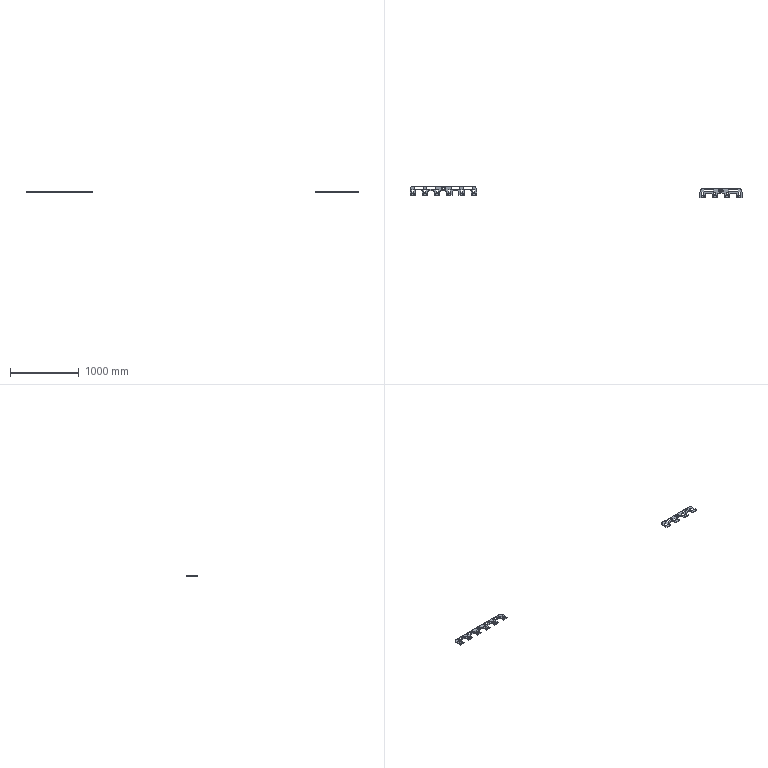NC program | NX | posted with a generic post | part box 4825 x 168.213 x 13 mm
Lines 4335 to 5402 of 9095:
(HOLE_MILLING , TOOL : D6)
N8620 T06 M6
N8622 G54
N8624 G17 G0 G90 X-10.715 Y58.869 S9500 M3
N8626 G43 Z30. H6
N8628 Z0.5
N8630 G94 G3 X-10.215 Y58.369 R0.5 F1400.
N8632 X-9.715 Y58.869 R0.5
N8634 X-9.715 Y58.869 Z0. I-1. J0.
N8636 X-9.715 Y58.869 Z-0.5 I-1. J0.
N8638 X-9.715 Y58.869 Z-1. I-1. J0.
N8640 X-9.715 Y58.869 Z-1.5 I-1. J0.
N8642 X-9.715 Y58.869 Z-2. I-1. J0.
N8644 X-9.715 Y58.869 Z-2.5 I-1. J0.
N8646 X-9.715 Y58.869 Z-3. I-1. J0.
N8648 X-9.715 Y58.869 Z-3.5 I-1. J0.
N8650 X-9.715 Y58.869 Z-4. I-1. J0.
N8652 X-9.715 Y58.869 Z-4.5 I-1. J0.
N8654 X-10.406 Y59.82 Z-4.6 R1.
N8656 X-11.666 Y59.178 R1.
N8658 X-10.406 Y59.82 R-1.
N8660 X-11.036 Y59.499 R0.5
N8662 X-10.715 Y58.869 R0.5
N8664 G0 Z30.
N8666 X-25.869 Y43.715
N8668 Z0.5
N8670 G3 X-25.369 Y43.215 R0.5
N8672 X-24.869 Y43.715 R0.5
N8674 X-24.869 Y43.715 Z0. I-1. J0.
N8676 X-24.869 Y43.715 Z-0.5 I-1. J0.
N8678 X-24.869 Y43.715 Z-1. I-1. J0.
N8680 X-24.869 Y43.715 Z-1.5 I-1. J0.
N8682 X-24.869 Y43.715 Z-2. I-1. J0.
N8684 X-24.869 Y43.715 Z-2.5 I-1. J0.
N8686 X-24.869 Y43.715 Z-3. I-1. J0.
N8688 X-24.869 Y43.715 Z-3.5 I-1. J0.
N8690 X-24.869 Y43.715 Z-4. I-1. J0.
N8692 X-24.869 Y43.715 Z-4.5 I-1. J0.
N8694 X-25.56 Y44.666 Z-4.6 R1.
N8696 X-26.82 Y44.024 R1.
N8698 X-25.56 Y44.666 R-1.
N8700 X-26.19 Y44.345 R0.5
N8702 X-25.869 Y43.715 R0.5
N8704 G0 Z30.
N8706 Y22.285
N8708 Z0.5
N8710 G3 X-25.369 Y21.785 R0.5
N8712 X-24.869 Y22.285 R0.5
N8714 X-24.869 Y22.285 Z0. I-1. J0.
N8716 X-24.869 Y22.285 Z-0.5 I-1. J0.
N8718 X-24.869 Y22.285 Z-1. I-1. J0.
N8720 X-24.869 Y22.285 Z-1.5 I-1. J0.
N8722 X-24.869 Y22.285 Z-2. I-1. J0.
N8724 X-24.869 Y22.285 Z-2.5 I-1. J0.
N8726 X-24.869 Y22.285 Z-3. I-1. J0.
N8728 X-24.869 Y22.285 Z-3.5 I-1. J0.
N8730 X-24.869 Y22.285 Z-4. I-1. J0.
N8732 X-24.869 Y22.285 Z-4.5 I-1. J0.
N8734 X-25.56 Y23.236 Z-4.6 R1.
N8736 X-26.82 Y22.594 R1.
N8738 X-25.56 Y23.236 R-1.
N8740 X-26.19 Y22.915 R0.5
N8742 X-25.869 Y22.285 R0.5
N8744 G0 Z30.
N8746 X-10.715 Y7.131
N8748 Z0.5
N8750 G3 X-10.215 Y6.631 R0.5
N8752 X-9.715 Y7.131 R0.5
N8754 X-9.715 Y7.131 Z0. I-1. J0.
N8756 X-9.715 Y7.131 Z-0.5 I-1. J0.
N8758 X-9.715 Y7.131 Z-1. I-1. J0.
N8760 X-9.715 Y7.131 Z-1.5 I-1. J0.
N8762 X-9.715 Y7.131 Z-2. I-1. J0.
N8764 X-9.715 Y7.131 Z-2.5 I-1. J0.
N8766 X-9.715 Y7.131 Z-3. I-1. J0.
N8768 X-9.715 Y7.131 Z-3.5 I-1. J0.
N8770 X-9.715 Y7.131 Z-4. I-1. J0.
N8772 X-9.715 Y7.131 Z-4.5 I-1. J0.
N8774 X-10.406 Y8.082 Z-4.6 R1.
N8776 X-11.666 Y7.44 R1.
N8778 X-10.406 Y8.082 R-1.
N8780 X-11.036 Y7.761 R0.5
N8782 X-10.715 Y7.131 R0.5
N8784 G0 Z30.
N8786 X10.715
N8788 Z0.5
N8790 G3 X11.215 Y6.631 R0.5
N8792 X11.715 Y7.131 R0.5
N8794 X11.715 Y7.131 Z0. I-1. J0.
N8796 X11.715 Y7.131 Z-0.5 I-1. J0.
N8798 X11.715 Y7.131 Z-1. I-1. J0.
N8800 X11.715 Y7.131 Z-1.5 I-1. J0.
N8802 X11.715 Y7.131 Z-2. I-1. J0.
N8804 X11.715 Y7.131 Z-2.5 I-1. J0.
N8806 X11.715 Y7.131 Z-3. I-1. J0.
N8808 X11.715 Y7.131 Z-3.5 I-1. J0.
N8810 X11.715 Y7.131 Z-4. I-1. J0.
N8812 X11.715 Y7.131 Z-4.5 I-1. J0.
N8814 X11.024 Y8.082 Z-4.6 R1.
N8816 X9.764 Y7.44 R1.
N8818 X11.024 Y8.082 R-1.
N8820 X10.394 Y7.761 R0.5
N8822 X10.715 Y7.131 R0.5
N8824 G0 Z30.
N8826 X25.869 Y22.285
N8828 Z0.5
N8830 G3 X26.369 Y21.785 R0.5
N8832 X26.869 Y22.285 R0.5
N8834 X26.869 Y22.285 Z0. I-1. J0.
N8836 X26.869 Y22.285 Z-0.5 I-1. J0.
N8838 X26.869 Y22.285 Z-1. I-1. J0.
N8840 X26.869 Y22.285 Z-1.5 I-1. J0.
N8842 X26.869 Y22.285 Z-2. I-1. J0.
N8844 X26.869 Y22.285 Z-2.5 I-1. J0.
N8846 X26.869 Y22.285 Z-3. I-1. J0.
N8848 X26.869 Y22.285 Z-3.5 I-1. J0.
N8850 X26.869 Y22.285 Z-4. I-1. J0.
N8852 X26.869 Y22.285 Z-4.5 I-1. J0.
N8854 X26.178 Y23.236 Z-4.6 R1.
N8856 X24.918 Y22.594 R1.
N8858 X26.178 Y23.236 R-1.
N8860 X25.548 Y22.915 R0.5
N8862 X25.869 Y22.285 R0.5
N8864 G0 Z30.
N8866 Y43.715
N8868 Z0.5
N8870 G3 X26.369 Y43.215 R0.5
N8872 X26.869 Y43.715 R0.5
N8874 X26.869 Y43.715 Z0. I-1. J0.
N8876 X26.869 Y43.715 Z-0.5 I-1. J0.
N8878 X26.869 Y43.715 Z-1. I-1. J0.
N8880 X26.869 Y43.715 Z-1.5 I-1. J0.
N8882 X26.869 Y43.715 Z-2. I-1. J0.
N8884 X26.869 Y43.715 Z-2.5 I-1. J0.
N8886 X26.869 Y43.715 Z-3. I-1. J0.
N8888 X26.869 Y43.715 Z-3.5 I-1. J0.
N8890 X26.869 Y43.715 Z-4. I-1. J0.
N8892 X26.869 Y43.715 Z-4.5 I-1. J0.
N8894 X26.178 Y44.666 Z-4.6 R1.
N8896 X24.918 Y44.024 R1.
N8898 X26.178 Y44.666 R-1.
N8900 X25.548 Y44.345 R0.5
N8902 X25.869 Y43.715 R0.5
N8904 G0 Z30.
N8906 X10.715 Y58.869
N8908 Z0.5
N8910 G3 X11.215 Y58.369 R0.5
N8912 X11.715 Y58.869 R0.5
N8914 X11.715 Y58.869 Z0. I-1. J0.
N8916 X11.715 Y58.869 Z-0.5 I-1. J0.
N8918 X11.715 Y58.869 Z-1. I-1. J0.
N8920 X11.715 Y58.869 Z-1.5 I-1. J0.
N8922 X11.715 Y58.869 Z-2. I-1. J0.
N8924 X11.715 Y58.869 Z-2.5 I-1. J0.
N8926 X11.715 Y58.869 Z-3. I-1. J0.
N8928 X11.715 Y58.869 Z-3.5 I-1. J0.
N8930 X11.715 Y58.869 Z-4. I-1. J0.
N8932 X11.715 Y58.869 Z-4.5 I-1. J0.
N8934 X11.024 Y59.82 Z-4.6 R1.
N8936 X9.764 Y59.178 R1.
N8938 X11.024 Y59.82 R-1.
N8940 X10.394 Y59.499 R0.5
N8942 X10.715 Y58.869 R0.5
N8944 G0 Z30.
(ZLEVEL_PROFILE_COPY_1 , TOOL : D6)
N8946 X276.421 Y-19.8
N8948 Z-0.591
N8950 G1 Y-20.997 F1000.
N8952 X276.484 Y-21.
N8954 X278.7 F1650.
N8956 Y-18.784
N8958 X278.697 Y-18.721
N8960 X277.5
N8962 G0 X276.421 Y-19.8 Z-1.182
N8964 G1 Y-20.997 F1000.
N8966 X276.484 Y-21.
N8968 X278.7 F1650.
N8970 Y-18.784
N8972 X278.697 Y-18.721
N8974 X277.5
N8976 G0 X276.421 Y-19.8 Z-1.773
N8978 G1 Y-20.997 F1000.
N8980 X276.484 Y-21.
N8982 X278.7 F1650.
N8984 Y-18.784
N8986 X278.697 Y-18.721
N8988 X277.5
N8990 G0 X276.421 Y-19.8 Z-2.364
N8992 G1 Y-20.997 F1000.
N8994 X276.484 Y-21.
N8996 X278.7 F1650.
N8998 Y-18.784
N9000 X278.697 Y-18.721
N9002 X277.5
N9004 G0 X276.421 Y-19.8 Z-2.955
N9006 G1 Y-20.997 F1000.
N9008 X276.484 Y-21.
N9010 X278.7 F1650.
N9012 Y-18.784
N9014 X278.697 Y-18.721
N9016 X277.5
N9018 G0 X276.421 Y-19.8 Z-3.545
N9020 G1 Y-20.997 F1000.
N9022 X276.484 Y-21.
N9024 X278.7 F1650.
N9026 Y-18.784
N9028 X278.697 Y-18.721
N9030 X277.5
N9032 G0 X276.421 Y-19.8 Z-4.136
N9034 G1 Y-20.997 F1000.
N9036 X276.484 Y-21.
N9038 X278.7 F1650.
N9040 Y-18.784
N9042 X278.697 Y-18.721
N9044 X277.5
N9046 G0 X276.421 Y-19.8 Z-4.727
N9048 G1 Y-20.997 F1000.
N9050 X276.484 Y-21.
N9052 X278.7 F1650.
N9054 Y-18.784
N9056 X278.697 Y-18.721
N9058 X277.5
N9060 G0 X276.421 Y-19.8 Z-5.318
N9062 G1 Y-20.997 F1000.
N9064 X276.484 Y-21.
N9066 X278.7 F1650.
N9068 Y-18.784
N9070 X278.697 Y-18.721
N9072 X277.5
N9074 G0 X276.421 Y-19.8 Z-5.909
N9076 G1 Y-20.997 F1000.
N9078 X276.484 Y-21.
N9080 X278.7 F1650.
N9082 Y-18.784
N9084 X278.697 Y-18.721
N9086 X277.5
N9088 G0 X276.421 Y-19.8 Z-6.5
N9090 G1 Y-20.997 F1000.
N9092 X276.484 Y-21.
N9094 X278.7 F1650.
N9096 Y-18.784
N9098 X278.697 Y-18.721
N9100 X277.5
N9102 G0 X276.421 Y-19.8 Z-7.091
N9104 G1 Y-20.997 F1000.
N9106 X276.484 Y-21.
N9108 X278.7 F1650.
N9110 Y-18.784
N9112 X278.697 Y-18.721
N9114 X277.5
N9116 G0 X276.421 Y-19.8 Z-7.682
N9118 G1 Y-20.997 F1000.
N9120 X276.484 Y-21.
N9122 X278.7 F1650.
N9124 Y-18.784
N9126 X278.697 Y-18.721
N9128 X277.5
N9130 G0 X276.416 Y-19.8 Z-8.273
N9132 G1 Y-20.997 F1000.
N9134 X276.479 Y-21.
N9136 X278.7 F1650.
N9138 Y-18.783
N9140 X278.697 Y-18.72
N9142 X277.5
N9144 G0 X276.416 Y-19.8 Z-8.864
N9146 G1 Y-20.997 F1000.
N9148 X276.479 Y-21.
N9150 X278.7 F1650.
N9152 Y-18.783
N9154 X278.697 Y-18.72
N9156 X277.5
N9158 G0 X276.416 Y-19.8 Z-9.455
N9160 G1 Y-20.997 F1000.
N9162 X276.479 Y-21.
N9164 X278.7 F1650.
N9166 Y-18.783
N9168 X278.697 Y-18.72
N9170 X277.5
N9172 G0 X276.416 Y-19.8 Z-10.045
N9174 G1 Y-20.997 F1000.
N9176 X276.479 Y-21.
N9178 X278.7 F1650.
N9180 Y-18.783
N9182 X278.697 Y-18.72
N9184 X277.5
N9186 G0 X276.416 Y-19.8 Z-10.636
N9188 G1 Y-20.997 F1000.
N9190 X276.479 Y-21.
N9192 X278.7 F1650.
N9194 Y-18.783
N9196 X278.697 Y-18.72
N9198 X277.5
N9200 G0 X276.416 Y-19.8 Z-11.227
N9202 G1 Y-20.997 F1000.
N9204 X276.479 Y-21.
N9206 X278.7 F1650.
N9208 Y-18.783
N9210 X278.697 Y-18.72
N9212 X277.5
N9214 G0 X276.416 Y-19.8 Z-11.818
N9216 G1 Y-20.997 F1000.
N9218 X276.479 Y-21.
N9220 X278.7 F1650.
N9222 Y-18.783
N9224 X278.697 Y-18.72
N9226 X277.5
N9228 G0 X276.416 Y-19.8 Z-12.409
N9230 G1 Y-20.997 F1000.
N9232 X276.479 Y-21.
N9234 X278.7 F1650.
N9236 Y-18.783
N9238 X278.697 Y-18.72
N9240 X277.5
N9242 G0 X276.416 Y-19.8 Z-13.
N9244 G1 Y-20.997 F1000.
N9246 X276.479 Y-21.
N9248 X278.7 F1650.
N9250 Y-18.783
N9252 X278.697 Y-18.72
N9254 X277.5
N9256 G0 Z30.
N9258 Y10.721
N9260 Z-0.591
N9262 G1 X278.697 F1000.
N9264 X278.7 Y10.784
N9266 Y13. F1650.
N9268 X276.484
N9270 X276.421 Y12.997
N9272 Y11.8
N9274 G0 X277.5 Y10.721 Z-1.182
N9276 G1 X278.697 F1000.
N9278 X278.7 Y10.784
N9280 Y13. F1650.
N9282 X276.484
N9284 X276.421 Y12.997
N9286 Y11.8
N9288 G0 X277.5 Y10.721 Z-1.773
N9290 G1 X278.697 F1000.
N9292 X278.7 Y10.784
N9294 Y13. F1650.
N9296 X276.484
N9298 X276.421 Y12.997
N9300 Y11.8
N9302 G0 X277.5 Y10.721 Z-2.364
N9304 G1 X278.697 F1000.
N9306 X278.7 Y10.784
N9308 Y13. F1650.
N9310 X276.484
N9312 X276.421 Y12.997
N9314 Y11.8
N9316 G0 X277.5 Y10.721 Z-2.955
N9318 G1 X278.697 F1000.
N9320 X278.7 Y10.784
N9322 Y13. F1650.
N9324 X276.484
N9326 X276.421 Y12.997
N9328 Y11.8
N9330 G0 X277.5 Y10.721 Z-3.545
N9332 G1 X278.697 F1000.
N9334 X278.7 Y10.784
N9336 Y13. F1650.
N9338 X276.484
N9340 X276.421 Y12.997
N9342 Y11.8
N9344 G0 X277.5 Y10.721 Z-4.136
N9346 G1 X278.697 F1000.
N9348 X278.7 Y10.784
N9350 Y13. F1650.
N9352 X276.484
N9354 X276.421 Y12.997
N9356 Y11.8
N9358 G0 X277.5 Y10.721 Z-4.727
N9360 G1 X278.697 F1000.
N9362 X278.7 Y10.784
N9364 Y13. F1650.
N9366 X276.484
N9368 X276.421 Y12.997
N9370 Y11.8
N9372 G0 X277.5 Y10.721 Z-5.318
N9374 G1 X278.697 F1000.
N9376 X278.7 Y10.784
N9378 Y13. F1650.
N9380 X276.484
N9382 X276.421 Y12.997
N9384 Y11.8
N9386 G0 X277.5 Y10.721 Z-5.909
N9388 G1 X278.697 F1000.
N9390 X278.7 Y10.784
N9392 Y13. F1650.
N9394 X276.484
N9396 X276.421 Y12.997
N9398 Y11.8
N9400 G0 X277.5 Y10.721 Z-6.5
N9402 G1 X278.697 F1000.
N9404 X278.7 Y10.784
N9406 Y13. F1650.
N9408 X276.484
N9410 X276.421 Y12.997
N9412 Y11.8
N9414 G0 X277.5 Y10.721 Z-7.091
N9416 G1 X278.697 F1000.
N9418 X278.7 Y10.784
N9420 Y13. F1650.
N9422 X276.484
N9424 X276.421 Y12.997
N9426 Y11.8
N9428 G0 X277.5 Y10.721 Z-7.682
N9430 G1 X278.697 F1000.
N9432 X278.7 Y10.784
N9434 Y13. F1650.
N9436 X276.484
N9438 X276.421 Y12.997
N9440 Y11.8
N9442 G0 X277.5 Y10.722 Z-8.273
N9444 G1 X278.697 F1000.
N9446 X278.7 Y10.785
N9448 Y12.991 F1650.
N9450 Y13.
N9452 X276.492
N9454 X276.429 Y12.997
N9456 Y11.8
N9458 G0 X277.5 Y10.722 Z-8.864
N9460 G1 X278.697 F1000.
N9462 X278.7 Y10.785
N9464 Y12.991 F1650.
N9466 Y13.
N9468 X276.492
N9470 X276.429 Y12.997
N9472 Y11.8
N9474 G0 X277.5 Y10.722 Z-9.455
N9476 G1 X278.697 F1000.
N9478 X278.7 Y10.785
N9480 Y12.991 F1650.
N9482 Y13.
N9484 X276.492
N9486 X276.429 Y12.997
N9488 Y11.8
N9490 G0 X277.5 Y10.722 Z-10.045
N9492 G1 X278.697 F1000.
N9494 X278.7 Y10.785
N9496 Y12.991 F1650.
N9498 Y13.
N9500 X276.492
N9502 X276.429 Y12.997
N9504 Y11.8
N9506 G0 X277.5 Y10.722 Z-10.636
N9508 G1 X278.697 F1000.
N9510 X278.7 Y10.785
N9512 Y12.991 F1650.
N9514 Y13.
N9516 X276.492
N9518 X276.429 Y12.997
N9520 Y11.8
N9522 G0 X277.5 Y10.722 Z-11.227
N9524 G1 X278.697 F1000.
N9526 X278.7 Y10.785
N9528 Y12.991 F1650.
N9530 Y13.
N9532 X276.492
N9534 X276.429 Y12.997
N9536 Y11.8
N9538 G0 X277.5 Y10.722 Z-11.818
N9540 G1 X278.697 F1000.
N9542 X278.7 Y10.785
N9544 Y12.991 F1650.
N9546 Y13.
N9548 X276.492
N9550 X276.429 Y12.997
N9552 Y11.8
N9554 G0 X277.5 Y10.722 Z-12.409
N9556 G1 X278.697 F1000.
N9558 X278.7 Y10.785
N9560 Y12.991 F1650.
N9562 Y13.
N9564 X276.492
N9566 X276.429 Y12.997
N9568 Y11.8
N9570 G0 X277.5 Y10.722 Z-13.
N9572 G1 X278.697 F1000.
N9574 X278.7 Y10.785
N9576 Y12.991 F1650.
N9578 Y13.
N9580 X276.492
N9582 X276.429 Y12.997
N9584 Y11.8
N9586 G0 Z30.
N9588 X256.979
N9590 Z-0.591
N9592 G1 Y12.997 F1000.
N9594 X256.916 Y13.
N9596 X254.7 F1650.
N9598 Y10.784
N9600 X254.703 Y10.721
N9602 X255.9
N9604 G0 X256.979 Y11.8 Z-1.182
N9606 G1 Y12.997 F1000.
N9608 X256.916 Y13.
N9610 X254.7 F1650.
N9612 Y10.784
N9614 X254.703 Y10.721
N9616 X255.9
N9618 G0 X256.979 Y11.8 Z-1.773
N9620 G1 Y12.997 F1000.
N9622 X256.916 Y13.
N9624 X254.7 F1650.
N9626 Y10.784
N9628 X254.703 Y10.721
N9630 X255.9
N9632 G0 X256.979 Y11.8 Z-2.364
N9634 G1 Y12.997 F1000.
N9636 X256.916 Y13.
N9638 X254.7 F1650.
N9640 Y10.784
N9642 X254.703 Y10.721
N9644 X255.9
N9646 G0 X256.979 Y11.8 Z-2.955
N9648 G1 Y12.997 F1000.
N9650 X256.916 Y13.
N9652 X254.7 F1650.
N9654 Y10.784
N9656 X254.703 Y10.721
N9658 X255.9
N9660 G0 X256.979 Y11.8 Z-3.545
N9662 G1 Y12.997 F1000.
N9664 X256.916 Y13.
N9666 X254.7 F1650.
N9668 Y10.784
N9670 X254.703 Y10.721
N9672 X255.9
N9674 G0 X256.979 Y11.8 Z-4.136
N9676 G1 Y12.997 F1000.
N9678 X256.916 Y13.
N9680 X254.7 F1650.
N9682 Y10.784
N9684 X254.703 Y10.721
N9686 X255.9
N9688 G0 X256.979 Y11.8 Z-4.727
N9690 G1 Y12.997 F1000.
N9692 X256.916 Y13.
N9694 X254.7 F1650.
N9696 Y10.784
N9698 X254.703 Y10.721
N9700 X255.9
N9702 G0 X256.979 Y11.8 Z-5.318
N9704 G1 Y12.997 F1000.
N9706 X256.916 Y13.
N9708 X254.7 F1650.
N9710 Y10.784
N9712 X254.703 Y10.721
N9714 X255.9
N9716 G0 X256.979 Y11.8 Z-5.909
N9718 G1 Y12.997 F1000.
N9720 X256.916 Y13.
N9722 X254.7 F1650.
N9724 Y10.784
N9726 X254.703 Y10.721
N9728 X255.9
N9730 G0 X256.979 Y11.8 Z-6.5
N9732 G1 Y12.997 F1000.
N9734 X256.916 Y13.
N9736 X254.7 F1650.
N9738 Y10.784
N9740 X254.703 Y10.721
N9742 X255.9
N9744 G0 X256.979 Y11.8 Z-7.091
N9746 G1 Y12.997 F1000.
N9748 X256.916 Y13.
N9750 X254.7 F1650.
N9752 Y10.784
N9754 X254.703 Y10.721
N9756 X255.9
N9758 G0 X256.979 Y11.8 Z-7.682
N9760 G1 Y12.997 F1000.
N9762 X256.916 Y13.
N9764 X254.7 F1650.
N9766 Y10.784
N9768 X254.703 Y10.721
N9770 X255.9
N9772 G0 X256.966 Y11.8 Z-8.273
N9774 G1 Y12.997 F1000.
N9776 X256.904 Y13.
N9778 X254.7 F1650.
N9780 Y10.785
N9782 X254.703 Y10.723
N9784 X255.9
N9786 G0 X256.966 Y11.8 Z-8.864
N9788 G1 Y12.997 F1000.
N9790 X256.904 Y13.
N9792 X254.7 F1650.
N9794 Y10.785
N9796 X254.703 Y10.723
N9798 X255.9
N9800 G0 X256.966 Y11.8 Z-9.455
N9802 G1 Y12.997 F1000.
N9804 X256.904 Y13.
N9806 X254.7 F1650.
N9808 Y10.785
N9810 X254.703 Y10.723
N9812 X255.9
N9814 G0 X256.966 Y11.8 Z-10.045
N9816 G1 Y12.997 F1000.
N9818 X256.904 Y13.
N9820 X254.7 F1650.
N9822 Y10.785
N9824 X254.703 Y10.723
N9826 X255.9
N9828 G0 X256.966 Y11.8 Z-10.636
N9830 G1 Y12.997 F1000.
N9832 X256.904 Y13.
N9834 X254.7 F1650.
N9836 Y10.785
N9838 X254.703 Y10.723
N9840 X255.9
N9842 G0 X256.966 Y11.8 Z-11.227
N9844 G1 Y12.997 F1000.
N9846 X256.904 Y13.
N9848 X254.7 F1650.
N9850 Y10.785
N9852 X254.703 Y10.723
N9854 X255.9
N9856 G0 X256.966 Y11.8 Z-11.818
N9858 G1 Y12.997 F1000.
N9860 X256.904 Y13.
N9862 X254.7 F1650.
N9864 Y10.785
N9866 X254.703 Y10.723
N9868 X255.9
N9870 G0 X256.966 Y11.8 Z-12.409
N9872 G1 Y12.997 F1000.
N9874 X256.904 Y13.
N9876 X254.7 F1650.
N9878 Y10.785
N9880 X254.703 Y10.723
N9882 X255.9
N9884 G0 X256.966 Y11.8 Z-13.
N9886 G1 Y12.997 F1000.
N9888 X256.904 Y13.
N9890 X254.7 F1650.
N9892 Y10.785
N9894 X254.703 Y10.723
N9896 X255.9
N9898 G0 Z30.
N9900 Y-18.721
N9902 Z-0.591
N9904 G1 X254.703 F1000.
N9906 X254.7 Y-18.784
N9908 Y-20.95 F1650.
N9910 X254.699 Y-21.001
N9912 X254.764 Y-21.
N9914 X256.916
N9916 X256.979 Y-20.997
N9918 Y-19.8
N9920 G0 X255.9 Y-18.721 Z-1.182
N9922 G1 X254.703 F1000.
N9924 X254.7 Y-18.784
N9926 Y-20.95 F1650.
N9928 X254.699 Y-21.001
N9930 X254.764 Y-21.
N9932 X256.916
N9934 X256.979 Y-20.997
N9936 Y-19.8
N9938 G0 X255.9 Y-18.721 Z-1.773
N9940 G1 X254.703 F1000.
N9942 X254.7 Y-18.784
N9944 Y-20.95 F1650.
N9946 X254.699 Y-21.001
N9948 X254.764 Y-21.
N9950 X256.916
N9952 X256.979 Y-20.997
N9954 Y-19.8
N9956 G0 X255.9 Y-18.721 Z-2.364
N9958 G1 X254.703 F1000.
N9960 X254.7 Y-18.784
N9962 Y-20.95 F1650.
N9964 X254.699 Y-21.001
N9966 X254.764 Y-21.
N9968 X256.916
N9970 X256.979 Y-20.997
N9972 Y-19.8
N9974 G0 X255.9 Y-18.721 Z-2.955
N9976 G1 X254.703 F1000.
N9978 X254.7 Y-18.784
N9980 Y-20.95 F1650.
N9982 X254.699 Y-21.001
N9984 X254.764 Y-21.
N9986 X256.916
N9988 X256.979 Y-20.997
N9990 Y-19.8
N9992 G0 X255.9 Y-18.721 Z-3.545
N9994 G1 X254.703 F1000.
N9996 X254.7 Y-18.784
N9998 Y-20.95 F1650.
N10000 X254.699 Y-21.001
N10002 X254.764 Y-21.
N10004 X256.916
N10006 X256.979 Y-20.997
N10008 Y-19.8
N10010 G0 X255.9 Y-18.721 Z-4.136
N10012 G1 X254.703 F1000.
N10014 X254.7 Y-18.784
N10016 Y-20.95 F1650.
N10018 X254.699 Y-21.001
N10020 X254.764 Y-21.
N10022 X256.916
N10024 X256.979 Y-20.997
N10026 Y-19.8
N10028 G0 X255.9 Y-18.721 Z-4.727
N10030 G1 X254.703 F1000.
N10032 X254.7 Y-18.784
N10034 Y-21. F1650.
N10036 X256.916
N10038 X256.979 Y-20.997
N10040 Y-19.8
N10042 G0 X255.9 Y-18.721 Z-5.318
N10044 G1 X254.703 F1000.
N10046 X254.7 Y-18.784
N10048 Y-21. F1650.
N10050 X256.916
N10052 X256.979 Y-20.997
N10054 Y-19.8
N10056 G0 X255.9 Y-18.721 Z-5.909
N10058 G1 X254.703 F1000.
N10060 X254.7 Y-18.784
N10062 Y-21. F1650.
N10064 X256.916
N10066 X256.979 Y-20.997
N10068 Y-19.8
N10070 G0 X255.9 Y-18.721 Z-6.5
N10072 G1 X254.703 F1000.
N10074 X254.7 Y-18.784
N10076 Y-21. F1650.
N10078 X256.916
N10080 X256.979 Y-20.997
N10082 Y-19.8
N10084 G0 X255.9 Y-18.721 Z-7.091
N10086 G1 X254.703 F1000.
N10088 X254.7 Y-18.784
N10090 Y-21. F1650.
N10092 X256.916
N10094 X256.979 Y-20.997
N10096 Y-19.8
N10098 G0 X255.9 Y-18.721 Z-7.682
N10100 G1 X254.703 F1000.
N10102 X254.7 Y-18.784
N10104 Y-21. F1650.
N10106 X256.916
N10108 X256.979 Y-20.997
N10110 Y-19.8
N10112 G0 X255.9 Y-18.721 Z-8.273
N10114 G1 X254.703 F1000.
N10116 X254.7 Y-18.784
N10118 Y-20.95 F1650.
N10120 Y-21.
N10122 X254.764
N10124 X256.916
N10126 X256.979 Y-20.997
N10128 Y-19.8
N10130 G0 X255.9 Y-18.721 Z-8.864
N10132 G1 X254.703 F1000.
N10134 X254.7 Y-18.784
N10136 Y-20.95 F1650.
N10138 Y-21.
N10140 X254.764
N10142 X256.916
N10144 X256.979 Y-20.997
N10146 Y-19.8
N10148 G0 X255.9 Y-18.721 Z-9.455
N10150 G1 X254.703 F1000.
N10152 X254.7 Y-18.784
N10154 Y-20.95 F1650.
N10156 Y-21.
N10158 X254.764
N10160 X256.916
N10162 X256.979 Y-20.997
N10164 Y-19.8
N10166 G0 X255.9 Y-18.721 Z-10.045
N10168 G1 X254.703 F1000.
N10170 X254.7 Y-18.784
N10172 Y-20.95 F1650.
N10174 Y-21.
N10176 X254.764
N10178 X256.916
N10180 X256.979 Y-20.997
N10182 Y-19.8
N10184 G0 X255.9 Y-18.721 Z-10.636
N10186 G1 X254.703 F1000.
N10188 X254.7 Y-18.784
N10190 Y-20.95 F1650.
N10192 Y-21.
N10194 X254.764
N10196 X256.916
N10198 X256.979 Y-20.997
N10200 Y-19.8
N10202 G0 X255.9 Y-18.721 Z-11.227
N10204 G1 X254.703 F1000.
N10206 X254.7 Y-18.784
N10208 Y-20.95 F1650.
N10210 Y-21.
N10212 X254.764
N10214 X256.916
N10216 X256.979 Y-20.997
N10218 Y-19.8
N10220 G0 X255.9 Y-18.721 Z-11.818
N10222 G1 X254.703 F1000.
N10224 X254.7 Y-18.784
N10226 Y-20.95 F1650.
N10228 Y-21.
N10230 X254.764
N10232 X256.916
N10234 X256.979 Y-20.997
N10236 Y-19.8
N10238 G0 X255.9 Y-18.721 Z-12.409
N10240 G1 X254.703 F1000.
N10242 X254.7 Y-18.784
N10244 Y-20.95 F1650.
N10246 Y-21.
N10248 X254.764
N10250 X256.916
N10252 X256.979 Y-20.997
N10254 Y-19.8
N10256 G0 X255.9 Y-18.721 Z-13.
N10258 G1 X254.703 F1000.
N10260 X254.7 Y-18.784
N10262 Y-20.95 F1650.
N10264 Y-21.
N10266 X254.764
N10268 X256.916
N10270 X256.979 Y-20.997
N10272 Y-19.8
N10274 G0 Z30.
N10276 X98.621
N10278 Z-0.591
N10280 G1 Y-20.997 F1000.
N10282 X98.684 Y-21.
N10284 X100.9 F1650.
N10286 Y-18.784
N10288 X100.897 Y-18.721
N10290 X99.7
N10292 G0 X98.621 Y-19.8 Z-1.182
N10294 G1 Y-20.997 F1000.
N10296 X98.684 Y-21.
N10298 X100.9 F1650.
N10300 Y-18.784
N10302 X100.897 Y-18.721
N10304 X99.7
N10306 G0 X98.621 Y-19.8 Z-1.773
N10308 G1 Y-20.997 F1000.
N10310 X98.684 Y-21.
N10312 X100.9 F1650.
N10314 Y-18.784
N10316 X100.897 Y-18.721
N10318 X99.7
N10320 G0 X98.621 Y-19.8 Z-2.364
N10322 G1 Y-20.997 F1000.
N10324 X98.684 Y-21.
N10326 X100.9 F1650.
N10328 Y-18.784
N10330 X100.897 Y-18.721
N10332 X99.7
N10334 G0 X98.621 Y-19.8 Z-2.955
N10336 G1 Y-20.997 F1000.
N10338 X98.684 Y-21.
N10340 X100.9 F1650.
N10342 Y-18.784
N10344 X100.897 Y-18.721
N10346 X99.7
N10348 G0 X98.621 Y-19.8 Z-3.545
N10350 G1 Y-20.997 F1000.
N10352 X98.684 Y-21.
N10354 X100.9 F1650.
N10356 Y-18.784
N10358 X100.897 Y-18.721
N10360 X99.7
N10362 G0 X98.621 Y-19.8 Z-4.136
N10364 G1 Y-20.997 F1000.
N10366 X98.684 Y-21.
N10368 X100.9 F1650.
N10370 Y-18.784
N10372 X100.897 Y-18.721
N10374 X99.7
N10376 G0 X98.621 Y-19.8 Z-4.727
N10378 G1 Y-20.997 F1000.
N10380 X98.684 Y-21.
N10382 X100.9 F1650.
N10384 Y-18.784
N10386 X100.897 Y-18.721
N10388 X99.7
N10390 G0 X98.621 Y-19.8 Z-5.318
N10392 G1 Y-20.997 F1000.
N10394 X98.684 Y-21.
N10396 X100.9 F1650.
N10398 Y-18.784
N10400 X100.897 Y-18.721
N10402 X99.7
N10404 G0 X98.621 Y-19.8 Z-5.909
N10406 G1 Y-20.997 F1000.
N10408 X98.684 Y-21.
N10410 X100.9 F1650.
N10412 Y-18.784
N10414 X100.897 Y-18.721
N10416 X99.7
N10418 G0 X98.621 Y-19.8 Z-6.5
N10420 G1 Y-20.997 F1000.
N10422 X98.684 Y-21.
N10424 X100.9 F1650.
N10426 Y-18.784
N10428 X100.897 Y-18.721
N10430 X99.7
N10432 G0 X98.621 Y-19.8 Z-7.091
N10434 G1 Y-20.997 F1000.
N10436 X98.684 Y-21.
N10438 X100.9 F1650.
N10440 Y-18.784
N10442 X100.897 Y-18.721
N10444 X99.7
N10446 G0 X98.621 Y-19.8 Z-7.682
N10448 G1 Y-20.997 F1000.
N10450 X98.684 Y-21.
N10452 X100.9 F1650.
N10454 Y-18.784
N10456 X100.897 Y-18.721
N10458 X99.7
N10460 G0 X98.62 Y-19.8 Z-8.273
N10462 G1 Y-20.997 F1000.
N10464 X98.683 Y-21.
N10466 X100.9 F1650.
N10468 Y-18.791
N10470 X100.897 Y-18.729
N10472 X99.7
N10474 G0 X98.62 Y-19.8 Z-8.864
N10476 G1 Y-20.997 F1000.
N10478 X98.683 Y-21.
N10480 X100.9 F1650.
N10482 Y-18.791
N10484 X100.897 Y-18.729
N10486 X99.7
N10488 G0 X98.62 Y-19.8 Z-9.455
N10490 G1 Y-20.997 F1000.
N10492 X98.683 Y-21.
N10494 X100.9 F1650.
N10496 Y-18.791
N10498 X100.897 Y-18.729
N10500 X99.7
N10502 G0 X98.62 Y-19.8 Z-10.045
N10504 G1 Y-20.997 F1000.
N10506 X98.683 Y-21.
N10508 X100.9 F1650.
N10510 Y-18.791
N10512 X100.897 Y-18.729
N10514 X99.7
N10516 G0 X98.62 Y-19.8 Z-10.636
N10518 G1 Y-20.997 F1000.
N10520 X98.683 Y-21.
N10522 X100.9 F1650.
N10524 Y-18.791
N10526 X100.897 Y-18.729
N10528 X99.7
N10530 G0 X98.62 Y-19.8 Z-11.227
N10532 G1 Y-20.997 F1000.
N10534 X98.683 Y-21.
N10536 X100.9 F1650.
N10538 Y-18.791
N10540 X100.897 Y-18.729
N10542 X99.7
N10544 G0 X98.62 Y-19.8 Z-11.818
N10546 G1 Y-20.997 F1000.
N10548 X98.683 Y-21.
N10550 X100.9 F1650.
N10552 Y-18.791
N10554 X100.897 Y-18.729
N10556 X99.7
N10558 G0 X98.62 Y-19.8 Z-12.409
N10560 G1 Y-20.997 F1000.
N10562 X98.683 Y-21.
N10564 X100.9 F1650.
N10566 Y-18.791
N10568 X100.897 Y-18.729
N10570 X99.7
N10572 G0 X98.62 Y-19.8 Z-13.
N10574 G1 Y-20.997 F1000.
N10576 X98.683 Y-21.
N10578 X100.9 F1650.
N10580 Y-18.791
N10582 X100.897 Y-18.729
N10584 X99.7
N10586 G0 Z30.
N10588 Y10.721
N10590 Z-0.591
N10592 G1 X100.897 F1000.
N10594 X100.9 Y10.784
N10596 Y13. F1650.
N10598 X98.684
N10600 X98.621 Y12.997
N10602 Y11.8
N10604 G0 X99.7 Y10.721 Z-1.182
N10606 G1 X100.897 F1000.
N10608 X100.9 Y10.784
N10610 Y13. F1650.
N10612 X98.684
N10614 X98.621 Y12.997
N10616 Y11.8
N10618 G0 X99.7 Y10.721 Z-1.773
N10620 G1 X100.897 F1000.
N10622 X100.9 Y10.784
N10624 Y13. F1650.
N10626 X98.684
N10628 X98.621 Y12.997
N10630 Y11.8
N10632 G0 X99.7 Y10.721 Z-2.364
N10634 G1 X100.897 F1000.
N10636 X100.9 Y10.784
N10638 Y13. F1650.
N10640 X98.684
N10642 X98.621 Y12.997
N10644 Y11.8
N10646 G0 X99.7 Y10.721 Z-2.955
N10648 G1 X100.897 F1000.
N10650 X100.9 Y10.784
N10652 Y13. F1650.
N10654 X98.684
N10656 X98.621 Y12.997
N10658 Y11.8
N10660 G0 X99.7 Y10.721 Z-3.545
N10662 G1 X100.897 F1000.
N10664 X100.9 Y10.784
N10666 Y13. F1650.
N10668 X98.684
N10670 X98.621 Y12.997
N10672 Y11.8
N10674 G0 X99.7 Y10.721 Z-4.136
N10676 G1 X100.897 F1000.
N10678 X100.9 Y10.784
N10680 Y13. F1650.
N10682 X98.684
N10684 X98.621 Y12.997
N10686 Y11.8
N10688 G0 X99.7 Y10.721 Z-4.727
N10690 G1 X100.897 F1000.
N10692 X100.9 Y10.784
N10694 Y13. F1650.
N10696 X98.684
N10698 X98.621 Y12.997
N10700 Y11.8
N10702 G0 X99.7 Y10.721 Z-5.318
N10704 G1 X100.897 F1000.
N10706 X100.9 Y10.784
N10708 Y13. F1650.
N10710 X98.684
N10712 X98.621 Y12.997
N10714 Y11.8
N10716 G0 X99.7 Y10.721 Z-5.909
N10718 G1 X100.897 F1000.
N10720 X100.9 Y10.784
N10722 Y13. F1650.
N10724 X98.684
N10726 X98.621 Y12.997
N10728 Y11.8
N10730 G0 X99.7 Y10.721 Z-6.5
N10732 G1 X100.897 F1000.
N10734 X100.9 Y10.784
N10736 Y13. F1650.
N10738 X98.684
N10740 X98.621 Y12.997
N10742 Y11.8